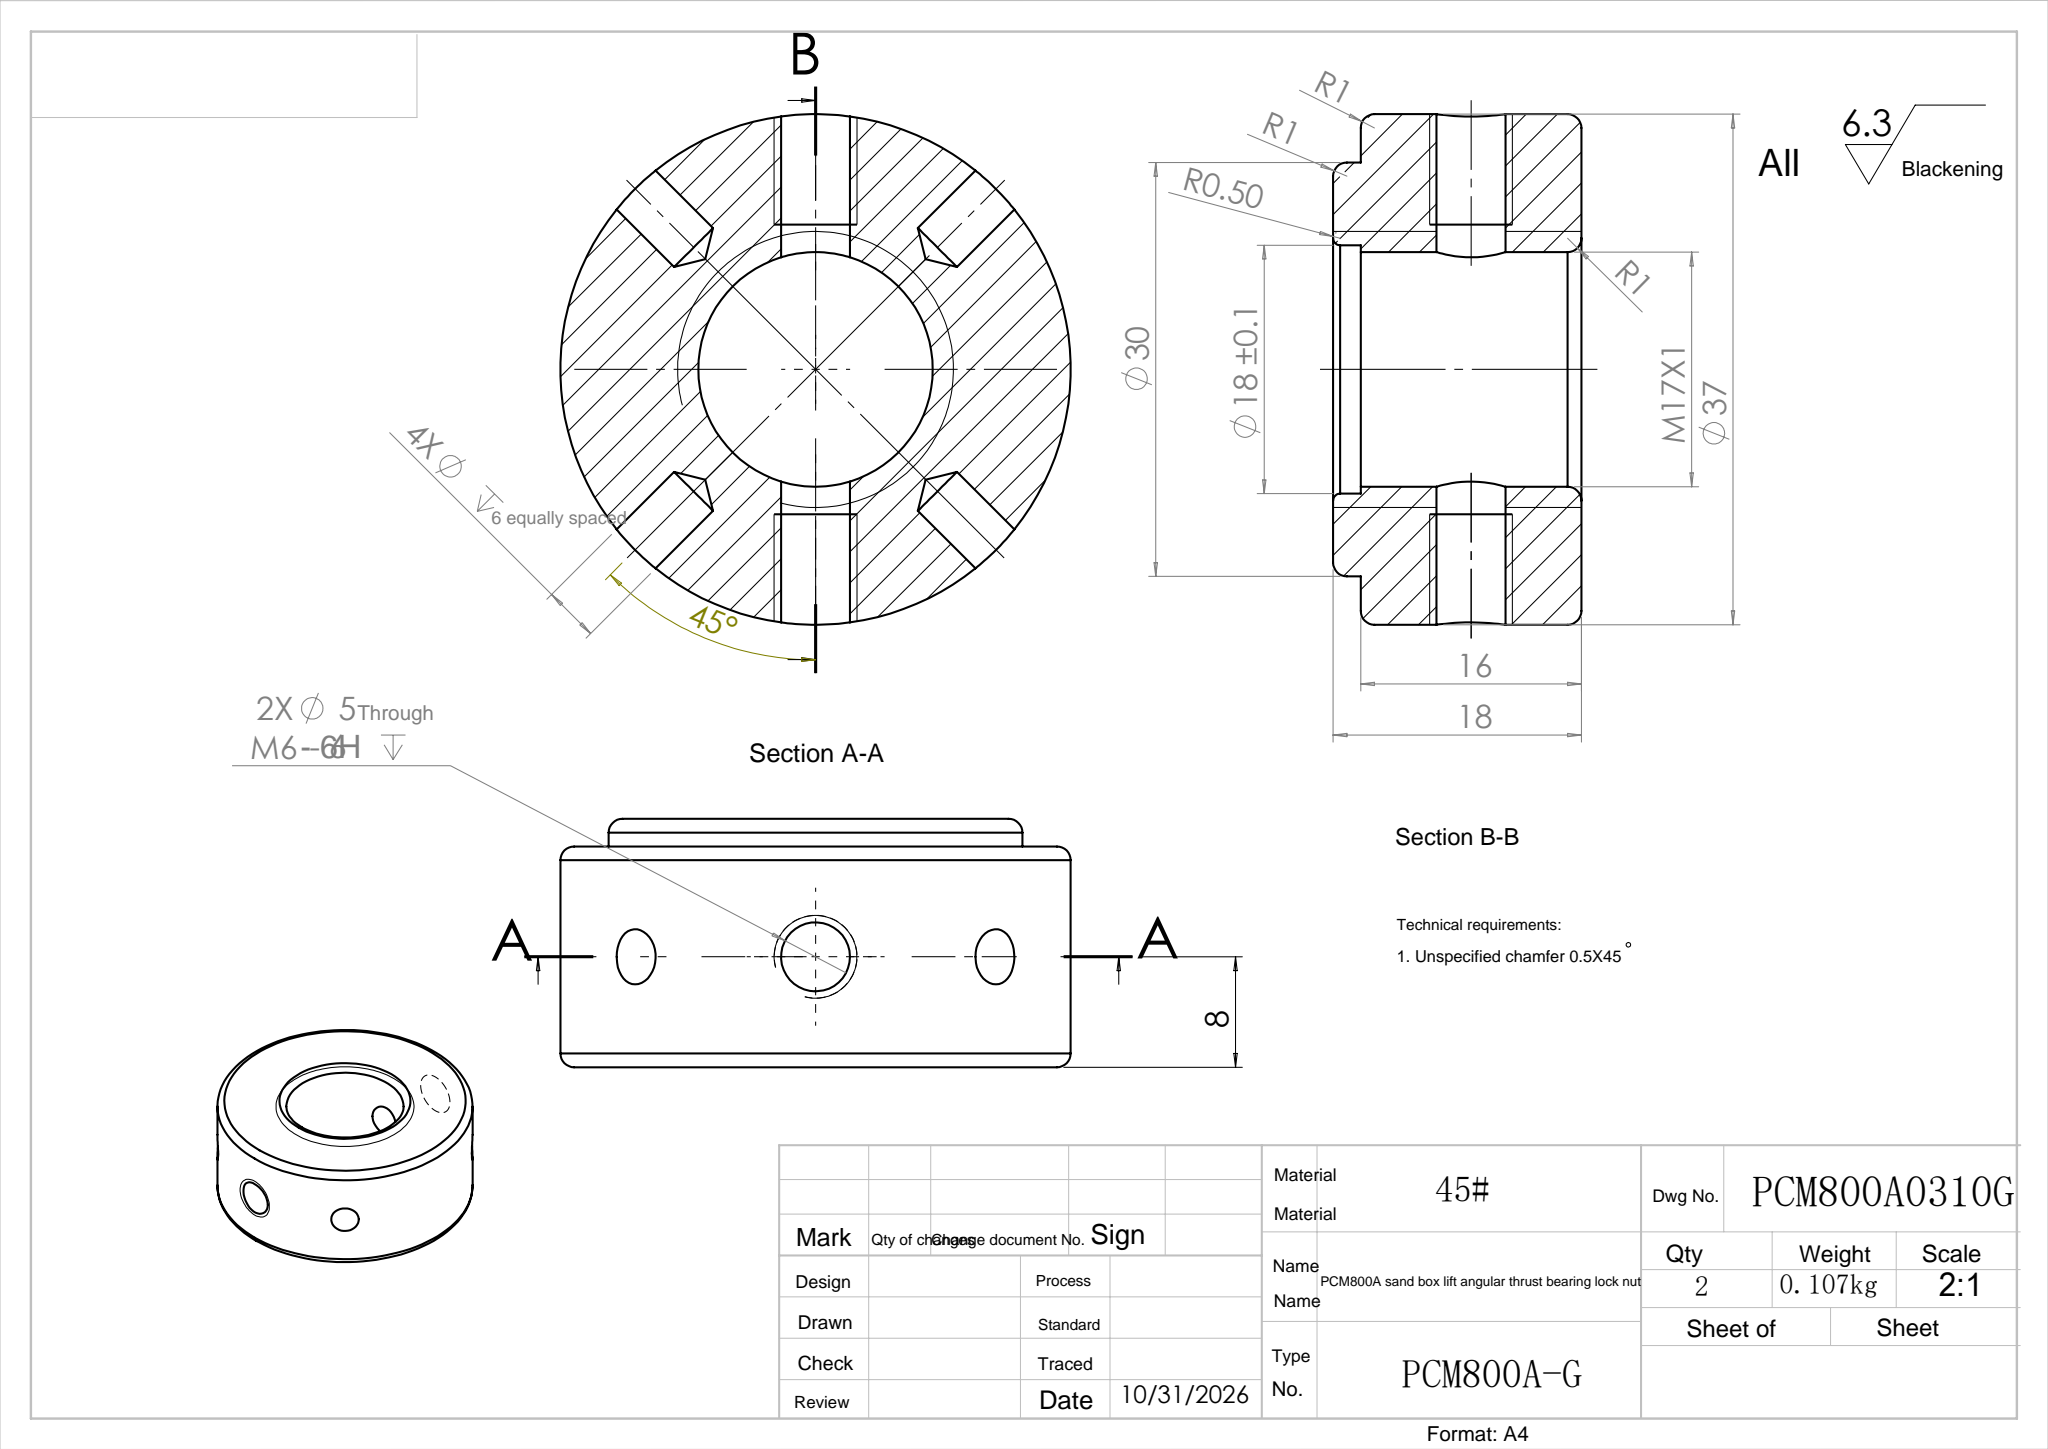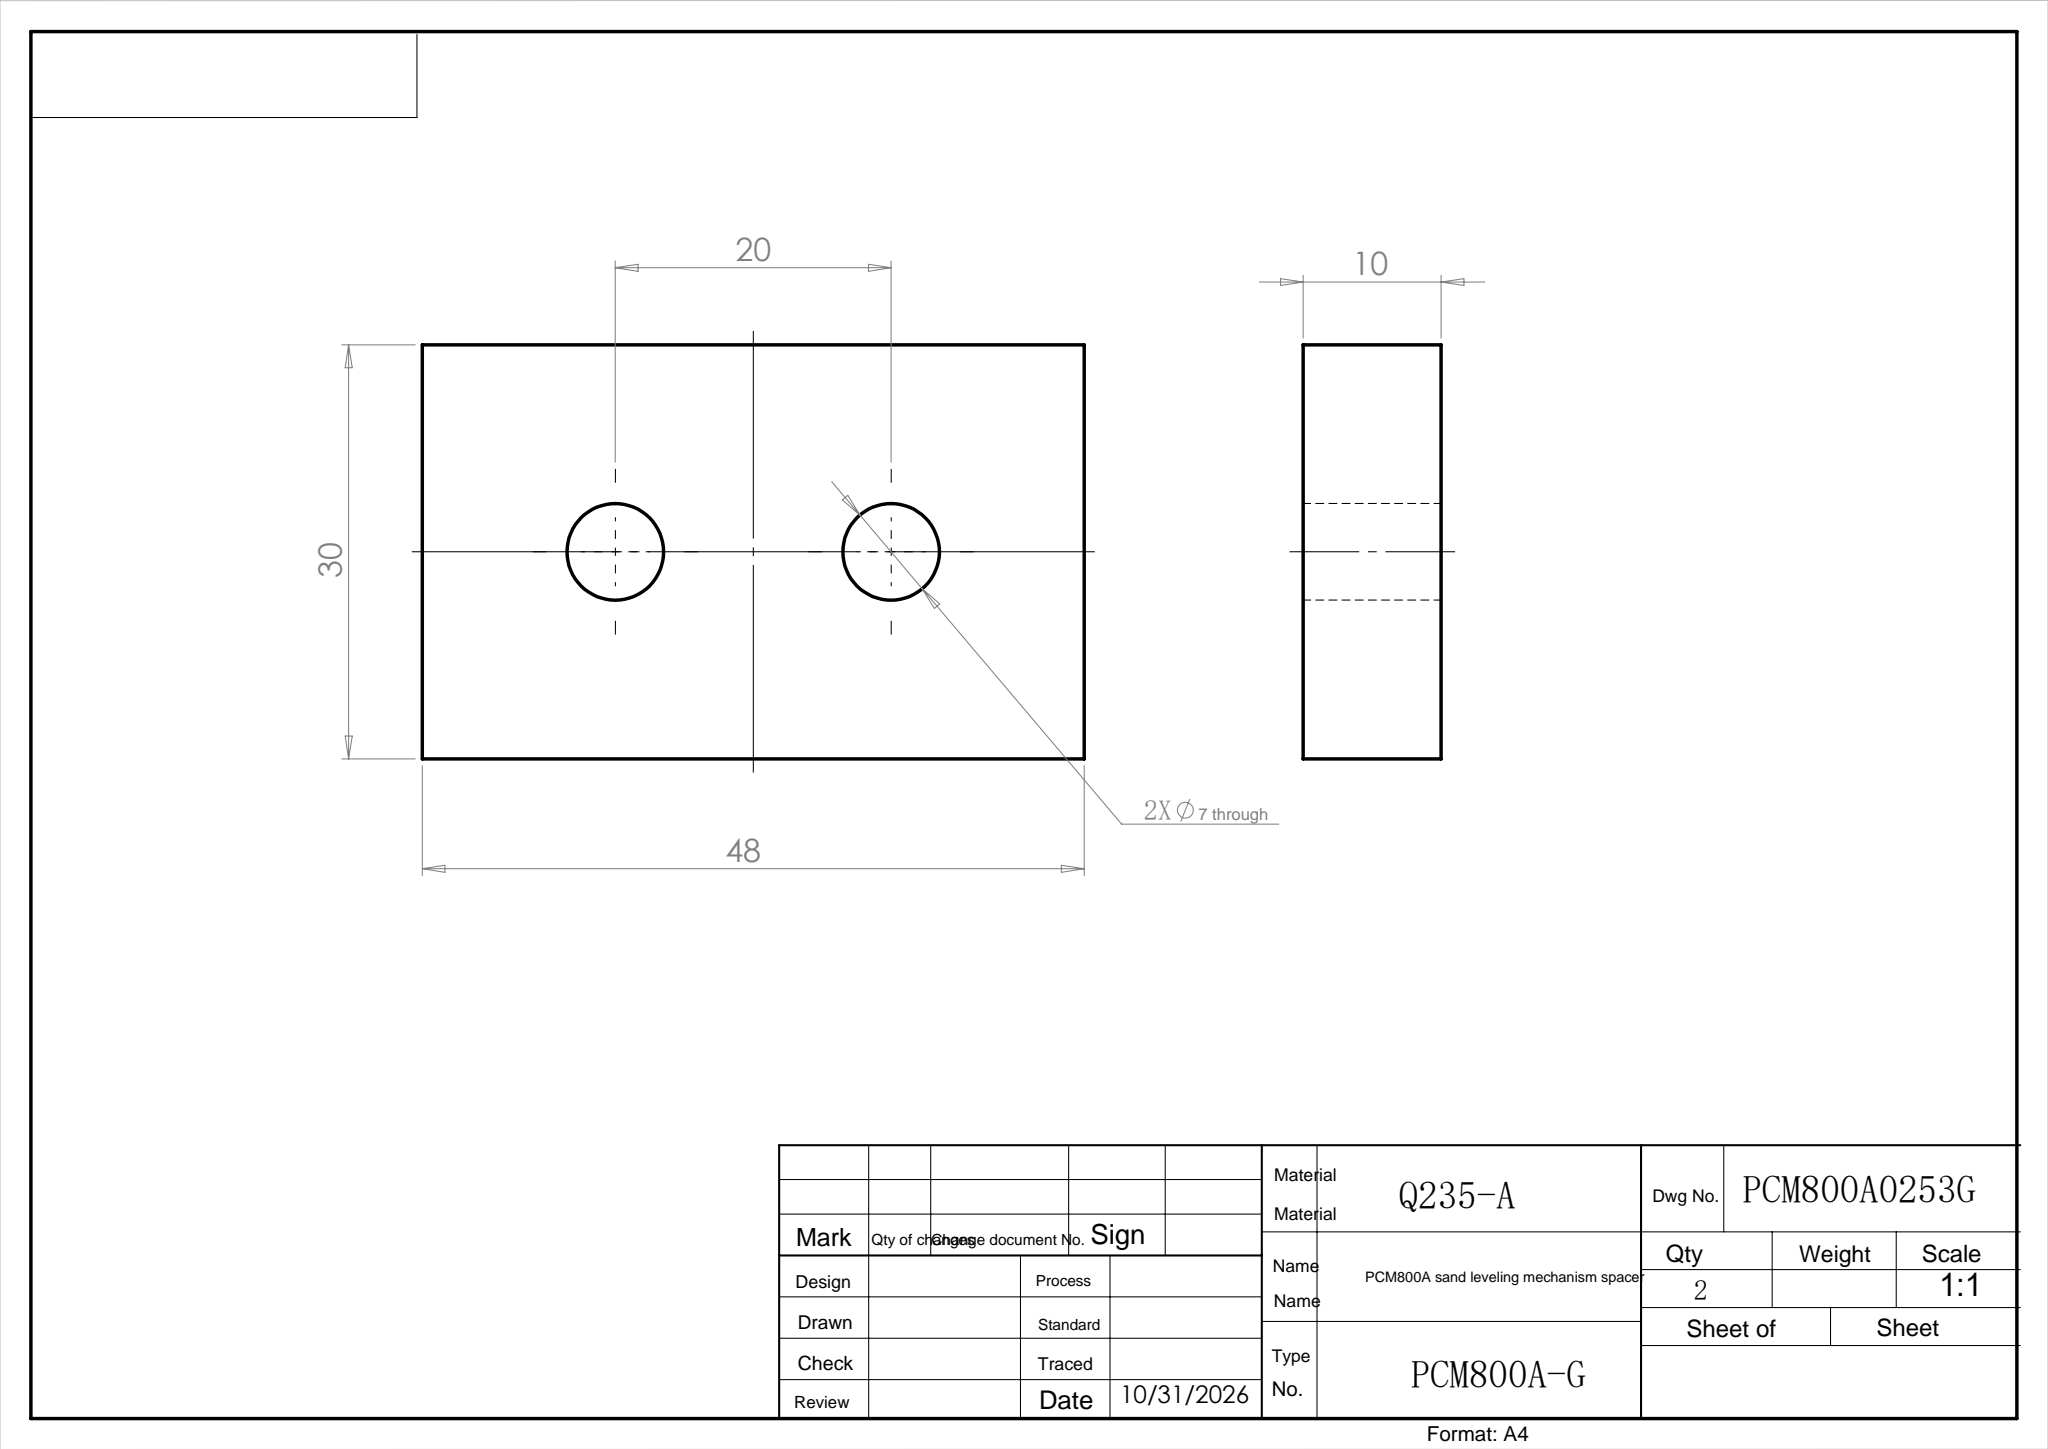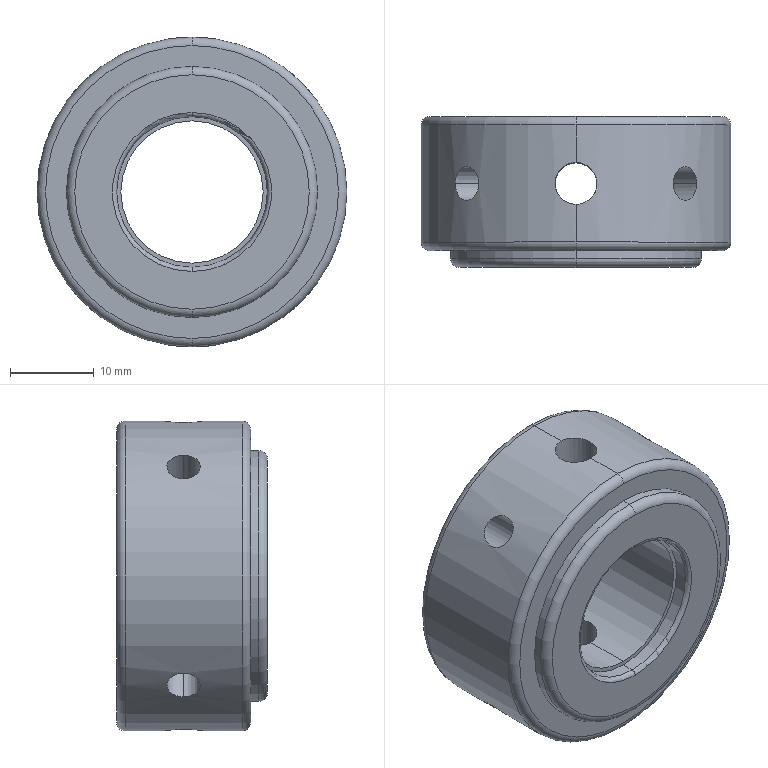Part | SolidWorks | features Fillet 3, HoleWzd 3, 3DProfileFeature 2, Boss 1, CirPattern 1, Cut 1, Extrusion 1, ICE 1 | 1 solid | 42 faces | box 37 x 18 x 37 mm | volume 13677 mm3 | cylinder 20 | torus 10 | cone 8 | plane 4 | commonest cylinder face diameters 4 x8 5 x4 17 x2 18 x2 30 x2 37 x2